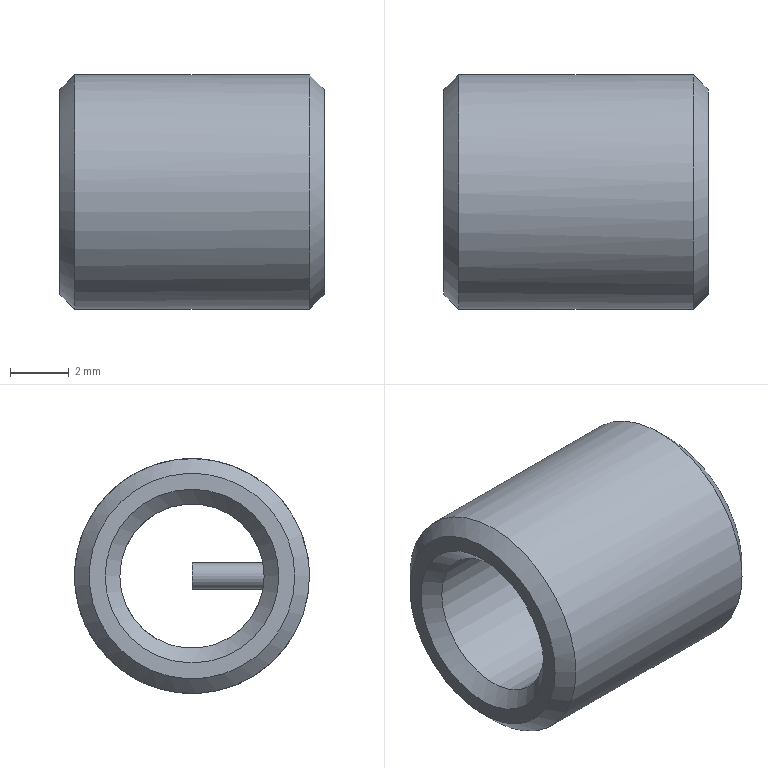Part | STEP file | Part [3] | 1 solid | 10 faces | box 9 x 8 x 8 mm | volume 272.983 mm3 | cone 4 | plane 3 | cylinder 3 | commonest cylinder face diameters 0.9 x1 4.917 x1 8 x1
STEP:
#1=CARTESIAN_POINT('',(13.5,104.,0.));
#2=VERTEX_POINT('',#1);
#3=CARTESIAN_POINT('',(13.5,107.5,0.));
#4=DIRECTION('',(1.,0.,0.));
#5=DIRECTION('',(0.,0.,1.));
#6=AXIS2_PLACEMENT_3D('',#3,#4,#5);
#7=CIRCLE('',#6,3.5);
#8=EDGE_CURVE('',#2,#2,#7,.T.);
#9=ORIENTED_EDGE('',*,*,#8,.F.);
#10=EDGE_LOOP('',(#9));
#11=FACE_BOUND('',#10,.T.);
#12=CARTESIAN_POINT('',(13.5,104.541,0.));
#13=VERTEX_POINT('',#12);
#14=CARTESIAN_POINT('',(13.5,107.5,0.));
#15=DIRECTION('',(1.,0.,0.));
#16=DIRECTION('',(0.,0.,1.));
#17=AXIS2_PLACEMENT_3D('',#14,#15,#16);
#18=CIRCLE('',#17,2.958);
#19=EDGE_CURVE('',#13,#13,#18,.T.);
#20=ORIENTED_EDGE('',*,*,#19,.T.);
#21=EDGE_LOOP('',(#20));
#22=FACE_BOUND('',#21,.T.);
#23=CARTESIAN_POINT('',(13.5,107.5,0.));
#24=DIRECTION('',(1.,0.,0.));
#25=DIRECTION('',(0.,0.,1.));
#26=AXIS2_PLACEMENT_3D('',#23,#24,#25);
#27=PLANE('',#26);
#28=ADVANCED_FACE('',(#11,#22),#27,.F.);
#29=CARTESIAN_POINT('',(14.,103.5,0.));
#30=VERTEX_POINT('',#29);
#31=CARTESIAN_POINT('',(14.,103.5,0.));
#32=CARTESIAN_POINT('',(14.,103.5,-0.08379));
#33=CARTESIAN_POINT('',(14.,103.505,-0.2514));
#34=CARTESIAN_POINT('',(14.,103.529,-0.5017));
#35=CARTESIAN_POINT('',(14.,103.568,-0.7501));
#36=CARTESIAN_POINT('',(14.,103.623,-0.9956));
#37=CARTESIAN_POINT('',(14.,103.693,-1.237));
#38=CARTESIAN_POINT('',(14.,103.779,-1.474));
#39=CARTESIAN_POINT('',(14.,103.878,-1.704));
#40=CARTESIAN_POINT('',(14.,103.993,-1.929));
#41=CARTESIAN_POINT('',(14.,104.121,-2.145));
#42=CARTESIAN_POINT('',(14.,104.262,-2.353));
#43=CARTESIAN_POINT('',(14.,104.416,-2.552));
#44=CARTESIAN_POINT('',(14.,104.583,-2.74));
#45=CARTESIAN_POINT('',(14.,104.76,-2.918));
#46=CARTESIAN_POINT('',(14.,104.949,-3.084));
#47=CARTESIAN_POINT('',(14.,105.148,-3.239));
#48=CARTESIAN_POINT('',(14.,105.356,-3.38));
#49=CARTESIAN_POINT('',(14.,105.572,-3.508));
#50=CARTESIAN_POINT('',(14.,105.796,-3.622));
#51=CARTESIAN_POINT('',(14.,106.027,-3.722));
#52=CARTESIAN_POINT('',(14.,106.264,-3.807));
#53=CARTESIAN_POINT('',(14.,106.505,-3.877));
#54=CARTESIAN_POINT('',(14.,106.751,-3.932));
#55=CARTESIAN_POINT('',(14.,106.999,-3.971));
#56=CARTESIAN_POINT('',(14.,107.25,-3.995));
#57=CARTESIAN_POINT('',(14.,107.501,-4.003));
#58=CARTESIAN_POINT('',(14.,107.752,-3.995));
#59=CARTESIAN_POINT('',(14.,108.003,-3.971));
#60=CARTESIAN_POINT('',(14.,108.251,-3.932));
#61=CARTESIAN_POINT('',(14.,108.497,-3.877));
#62=CARTESIAN_POINT('',(14.,108.738,-3.806));
#63=CARTESIAN_POINT('',(14.,108.975,-3.721));
#64=CARTESIAN_POINT('',(14.,109.205,-3.621));
#65=CARTESIAN_POINT('',(14.,109.429,-3.507));
#66=CARTESIAN_POINT('',(14.,109.646,-3.379));
#67=CARTESIAN_POINT('',(14.,109.854,-3.237));
#68=CARTESIAN_POINT('',(14.,110.052,-3.083));
#69=CARTESIAN_POINT('',(14.,110.241,-2.917));
#70=CARTESIAN_POINT('',(14.,110.419,-2.739));
#71=CARTESIAN_POINT('',(14.,110.585,-2.55));
#72=CARTESIAN_POINT('',(14.,110.739,-2.351));
#73=CARTESIAN_POINT('',(14.,110.88,-2.143));
#74=CARTESIAN_POINT('',(14.,111.008,-1.927));
#75=CARTESIAN_POINT('',(14.,111.122,-1.703));
#76=CARTESIAN_POINT('',(14.,111.222,-1.472));
#77=CARTESIAN_POINT('',(14.,111.307,-1.235));
#78=CARTESIAN_POINT('',(14.,111.377,-0.9936));
#79=CARTESIAN_POINT('',(14.,111.432,-0.7482));
#80=CARTESIAN_POINT('',(14.,111.471,-0.4998));
#81=CARTESIAN_POINT('',(14.,111.495,-0.25));
#82=CARTESIAN_POINT('',(14.,111.5,-0.08312));
#83=CARTESIAN_POINT('',(14.,111.5,0.));
#84=CARTESIAN_POINT('',(14.,111.5,0.08379));
#85=CARTESIAN_POINT('',(14.,111.495,0.2514));
#86=CARTESIAN_POINT('',(14.,111.471,0.5017));
#87=CARTESIAN_POINT('',(14.,111.432,0.7501));
#88=CARTESIAN_POINT('',(14.,111.377,0.9956));
#89=CARTESIAN_POINT('',(14.,111.307,1.237));
#90=CARTESIAN_POINT('',(14.,111.221,1.474));
#91=CARTESIAN_POINT('',(14.,111.122,1.704));
#92=CARTESIAN_POINT('',(14.,111.007,1.929));
#93=CARTESIAN_POINT('',(14.,110.879,2.145));
#94=CARTESIAN_POINT('',(14.,110.738,2.353));
#95=CARTESIAN_POINT('',(14.,110.584,2.552));
#96=CARTESIAN_POINT('',(14.,110.417,2.74));
#97=CARTESIAN_POINT('',(14.,110.24,2.918));
#98=CARTESIAN_POINT('',(14.,110.051,3.084));
#99=CARTESIAN_POINT('',(14.,109.852,3.239));
#100=CARTESIAN_POINT('',(14.,109.644,3.38));
#101=CARTESIAN_POINT('',(14.,109.428,3.508));
#102=CARTESIAN_POINT('',(14.,109.204,3.622));
#103=CARTESIAN_POINT('',(14.,108.973,3.722));
#104=CARTESIAN_POINT('',(14.,108.736,3.807));
#105=CARTESIAN_POINT('',(14.,108.495,3.877));
#106=CARTESIAN_POINT('',(14.,108.249,3.932));
#107=CARTESIAN_POINT('',(14.,108.001,3.971));
#108=CARTESIAN_POINT('',(14.,107.75,3.995));
#109=CARTESIAN_POINT('',(14.,107.499,4.003));
#110=CARTESIAN_POINT('',(14.,107.248,3.995));
#111=CARTESIAN_POINT('',(14.,106.997,3.971));
#112=CARTESIAN_POINT('',(14.,106.749,3.932));
#113=CARTESIAN_POINT('',(14.,106.503,3.877));
#114=CARTESIAN_POINT('',(14.,106.262,3.806));
#115=CARTESIAN_POINT('',(14.,106.025,3.721));
#116=CARTESIAN_POINT('',(14.,105.795,3.621));
#117=CARTESIAN_POINT('',(14.,105.571,3.507));
#118=CARTESIAN_POINT('',(14.,105.354,3.379));
#119=CARTESIAN_POINT('',(14.,105.146,3.237));
#120=CARTESIAN_POINT('',(14.,104.948,3.083));
#121=CARTESIAN_POINT('',(14.,104.759,2.917));
#122=CARTESIAN_POINT('',(14.,104.581,2.739));
#123=CARTESIAN_POINT('',(14.,104.415,2.55));
#124=CARTESIAN_POINT('',(14.,104.261,2.351));
#125=CARTESIAN_POINT('',(14.,104.12,2.143));
#126=CARTESIAN_POINT('',(14.,103.992,1.927));
#127=CARTESIAN_POINT('',(14.,103.878,1.703));
#128=CARTESIAN_POINT('',(14.,103.778,1.472));
#129=CARTESIAN_POINT('',(14.,103.693,1.235));
#130=CARTESIAN_POINT('',(14.,103.623,0.9936));
#131=CARTESIAN_POINT('',(14.,103.568,0.7482));
#132=CARTESIAN_POINT('',(14.,103.529,0.4998));
#133=CARTESIAN_POINT('',(14.,103.505,0.25));
#134=CARTESIAN_POINT('',(14.,103.5,0.08312));
#135=CARTESIAN_POINT('',(14.,103.5,0.));
#136=B_SPLINE_CURVE_WITH_KNOTS('',3,(#31,#32,#33,#34,#35,#36,#37,#38,#39,#40,#41,#42,#43,#44,#45,#46,#47,#48,#49,#50,#51,#52,#53,#54,#55,#56,#57,#58,#59,#60,#61,#62,#63,#64,#65,#66,#67,#68,#69,#70,#71,#72,#73,#74,#75,#76,#77,#78,#79,#80,#81,#82,#83,#84,#85,#86,#87,#88,#89,#90,#91,#92,#93,#94,#95,#96,#97,#98,#99,#100,#101,#102,#103,#104,#105,#106,#107,#108,#109,#110,#111,#112,#113,#114,#115,#116,#117,#118,#119,#120,#121,#122,#123,#124,#125,#126,#127,#128,#129,#130,#131,#132,#133,#134,#135),.UNSPECIFIED.,.T.,.F.,(4,1,1,1,1,1,1,1,1,1,1,1,1,1,1,1,1,1,1,1,1,1,1,1,1,1,1,1,1,1,1,1,1,1,1,1,1,1,1,1,1,1,1,1,1,1,1,1,1,1,3,1,1,1,1,1,1,1,1,1,1,1,1,1,1,1,1,1,1,1,1,1,1,1,1,1,1,1,1,1,1,1,1,1,1,1,1,1,1,1,1,1,1,1,1,1,1,1,1,1,4),(0.,0.01,0.02,0.03,0.04001,0.05001,0.06001,0.07001,0.08001,0.09001,0.1,0.11,0.12,0.13,0.14,0.15,0.16,0.17,0.18,0.19,0.2,0.21,0.22,0.23,0.24,0.25,0.26,0.27,0.28,0.29,0.3,0.31,0.3201,0.3301,0.3401,0.3501,0.3601,0.3701,0.3801,0.3901,0.4001,0.4101,0.4201,0.4301,0.4401,0.4501,0.4601,0.4701,0.4801,0.4901,0.5,0.51,0.52,0.53,0.54,0.55,0.56,0.57,0.58,0.59,0.6,0.61,0.62,0.63,0.64,0.65,0.66,0.67,0.68,0.69,0.7,0.71,0.72,0.73,0.74,0.75,0.76,0.77,0.78,0.79,0.8,0.81,0.8201,0.8301,0.8401,0.8501,0.8601,0.8701,0.8801,0.8901,0.9001,0.9101,0.9201,0.9301,0.9401,0.9501,0.9601,0.9701,0.9801,0.9901,1.),.UNSPECIFIED.);
#137=EDGE_CURVE('',#30,#30,#136,.T.);
#138=ORIENTED_EDGE('',*,*,#137,.F.);
#139=EDGE_LOOP('',(#138));
#140=FACE_OUTER_BOUND('',#139,.T.);
#141=ORIENTED_EDGE('',*,*,#8,.T.);
#142=EDGE_LOOP('',(#141));
#143=FACE_OUTER_BOUND('',#142,.T.);
#144=CARTESIAN_POINT('',(13.75,107.5,0.));
#145=DIRECTION('',(1.,0.,0.));
#146=DIRECTION('',(0.,-1.,0.));
#147=AXIS2_PLACEMENT_3D('',#144,#145,#146);
#148=CONICAL_SURFACE('',#147,3.75,0.7854);
#149=ADVANCED_FACE('',(#140,#143),#148,.T.);
#150=CARTESIAN_POINT('',(22.,103.5,0.));
#151=VERTEX_POINT('',#150);
#152=CARTESIAN_POINT('',(22.,111.5,0.));
#153=VERTEX_POINT('',#152);
#154=CARTESIAN_POINT('',(22.,107.5,0.));
#155=DIRECTION('',(1.,0.,0.));
#156=DIRECTION('',(0.,-1.,0.));
#157=AXIS2_PLACEMENT_3D('',#154,#155,#156);
#158=CIRCLE('',#157,4.);
#159=EDGE_CURVE('',#151,#153,#158,.T.);
#160=ORIENTED_EDGE('',*,*,#159,.F.);
#161=CARTESIAN_POINT('',(22.,107.5,0.));
#162=DIRECTION('',(1.,0.,0.));
#163=DIRECTION('',(0.,1.,0.));
#164=AXIS2_PLACEMENT_3D('',#161,#162,#163);
#165=CIRCLE('',#164,4.);
#166=EDGE_CURVE('',#153,#151,#165,.T.);
#167=ORIENTED_EDGE('',*,*,#166,.F.);
#168=EDGE_LOOP('',(#160,#167));
#169=FACE_BOUND('',#168,.T.);
#170=ORIENTED_EDGE('',*,*,#137,.T.);
#171=EDGE_LOOP('',(#170));
#172=FACE_OUTER_BOUND('',#171,.T.);
#173=CARTESIAN_POINT('',(13.5,107.5,0.));
#174=DIRECTION('',(1.,0.,0.));
#175=DIRECTION('',(0.,-1.,0.));
#176=AXIS2_PLACEMENT_3D('',#173,#174,#175);
#177=CYLINDRICAL_SURFACE('',#176,4.);
#178=ADVANCED_FACE('',(#169,#172),#177,.T.);
#179=CARTESIAN_POINT('',(22.5,111.,0.));
#180=VERTEX_POINT('',#179);
#181=CARTESIAN_POINT('',(22.5,107.5,0.));
#182=DIRECTION('',(1.,0.,0.));
#183=DIRECTION('',(0.,0.,1.));
#184=AXIS2_PLACEMENT_3D('',#181,#182,#183);
#185=CIRCLE('',#184,3.5);
#186=EDGE_CURVE('',#180,#180,#185,.T.);
#187=ORIENTED_EDGE('',*,*,#186,.F.);
#188=EDGE_LOOP('',(#187));
#189=FACE_OUTER_BOUND('',#188,.T.);
#190=ORIENTED_EDGE('',*,*,#166,.T.);
#191=ORIENTED_EDGE('',*,*,#159,.T.);
#192=EDGE_LOOP('',(#190,#191));
#193=FACE_BOUND('',#192,.T.);
#194=CARTESIAN_POINT('',(22.25,107.5,0.));
#195=DIRECTION('',(-1.,0.,0.));
#196=DIRECTION('',(0.,-1.,0.));
#197=AXIS2_PLACEMENT_3D('',#194,#195,#196);
#198=CONICAL_SURFACE('',#197,3.75,0.7854);
#199=ADVANCED_FACE('',(#189,#193),#198,.T.);
#200=ORIENTED_EDGE('',*,*,#186,.T.);
#201=EDGE_LOOP('',(#200));
#202=FACE_BOUND('',#201,.T.);
#203=CARTESIAN_POINT('',(22.5,104.541,0.));
#204=VERTEX_POINT('',#203);
#205=CARTESIAN_POINT('',(22.5,107.5,0.));
#206=DIRECTION('',(1.,0.,0.));
#207=DIRECTION('',(0.,0.,1.));
#208=AXIS2_PLACEMENT_3D('',#205,#206,#207);
#209=CIRCLE('',#208,2.958);
#210=EDGE_CURVE('',#204,#204,#209,.T.);
#211=ORIENTED_EDGE('',*,*,#210,.F.);
#212=EDGE_LOOP('',(#211));
#213=FACE_BOUND('',#212,.T.);
#214=CARTESIAN_POINT('',(22.5,107.5,0.));
#215=DIRECTION('',(1.,0.,0.));
#216=DIRECTION('',(0.,0.,1.));
#217=AXIS2_PLACEMENT_3D('',#214,#215,#216);
#218=PLANE('',#217);
#219=ADVANCED_FACE('',(#202,#213),#218,.T.);
#220=CARTESIAN_POINT('',(22.,105.083,-0.4472));
#221=VERTEX_POINT('',#220);
#222=CARTESIAN_POINT('',(22.,109.959,0.));
#223=VERTEX_POINT('',#222);
#224=CARTESIAN_POINT('',(22.,107.5,0.));
#225=DIRECTION('',(1.,0.,0.));
#226=DIRECTION('',(0.,-0.9833,-0.1819));
#227=AXIS2_PLACEMENT_3D('',#224,#225,#226);
#228=CIRCLE('',#227,2.458);
#229=EDGE_CURVE('',#221,#223,#228,.T.);
#230=ORIENTED_EDGE('',*,*,#229,.F.);
#231=CARTESIAN_POINT('',(22.5,104.541,0.));
#232=CARTESIAN_POINT('',(22.5,104.541,-0.002951));
#233=CARTESIAN_POINT('',(22.5,104.542,-0.009389));
#234=CARTESIAN_POINT('',(22.5,104.542,-0.01991));
#235=CARTESIAN_POINT('',(22.499,104.543,-0.03476));
#236=CARTESIAN_POINT('',(22.497,104.545,-0.0564));
#237=CARTESIAN_POINT('',(22.492,104.551,-0.08654));
#238=CARTESIAN_POINT('',(22.484,104.559,-0.1189));
#239=CARTESIAN_POINT('',(22.476,104.57,-0.1471));
#240=CARTESIAN_POINT('',(22.468,104.578,-0.1663));
#241=CARTESIAN_POINT('',(22.463,104.584,-0.1795));
#242=CARTESIAN_POINT('',(22.458,104.59,-0.1908));
#243=CARTESIAN_POINT('',(22.452,104.597,-0.2027));
#244=CARTESIAN_POINT('',(22.445,104.604,-0.2149));
#245=CARTESIAN_POINT('',(22.439,104.611,-0.2259));
#246=CARTESIAN_POINT('',(22.433,104.618,-0.2357));
#247=CARTESIAN_POINT('',(22.428,104.624,-0.2443));
#248=CARTESIAN_POINT('',(22.422,104.63,-0.2528));
#249=CARTESIAN_POINT('',(22.416,104.637,-0.2614));
#250=CARTESIAN_POINT('',(22.41,104.645,-0.2704));
#251=CARTESIAN_POINT('',(22.401,104.654,-0.2813));
#252=CARTESIAN_POINT('',(22.391,104.665,-0.2936));
#253=CARTESIAN_POINT('',(22.379,104.679,-0.3068));
#254=CARTESIAN_POINT('',(22.367,104.692,-0.3191));
#255=CARTESIAN_POINT('',(22.356,104.705,-0.3303));
#256=CARTESIAN_POINT('',(22.345,104.717,-0.3402));
#257=CARTESIAN_POINT('',(22.335,104.729,-0.3486));
#258=CARTESIAN_POINT('',(22.325,104.739,-0.3559));
#259=CARTESIAN_POINT('',(22.317,104.748,-0.3624));
#260=CARTESIAN_POINT('',(22.308,104.758,-0.3689));
#261=CARTESIAN_POINT('',(22.298,104.769,-0.3752));
#262=CARTESIAN_POINT('',(22.289,104.779,-0.3815));
#263=CARTESIAN_POINT('',(22.279,104.79,-0.3876));
#264=CARTESIAN_POINT('',(22.268,104.802,-0.3936));
#265=CARTESIAN_POINT('',(22.257,104.814,-0.3995));
#266=CARTESIAN_POINT('',(22.246,104.826,-0.4051));
#267=CARTESIAN_POINT('',(22.234,104.839,-0.4106));
#268=CARTESIAN_POINT('',(22.222,104.851,-0.4157));
#269=CARTESIAN_POINT('',(22.21,104.865,-0.4206));
#270=CARTESIAN_POINT('',(22.198,104.878,-0.4251));
#271=CARTESIAN_POINT('',(22.185,104.891,-0.4293));
#272=CARTESIAN_POINT('',(22.172,104.905,-0.4331));
#273=CARTESIAN_POINT('',(22.16,104.918,-0.4365));
#274=CARTESIAN_POINT('',(22.147,104.932,-0.4395));
#275=CARTESIAN_POINT('',(22.135,104.945,-0.442));
#276=CARTESIAN_POINT('',(22.123,104.957,-0.4441));
#277=CARTESIAN_POINT('',(22.111,104.97,-0.4459));
#278=CARTESIAN_POINT('',(22.1,104.981,-0.4473));
#279=CARTESIAN_POINT('',(22.089,104.993,-0.4484));
#280=CARTESIAN_POINT('',(22.078,105.004,-0.4492));
#281=CARTESIAN_POINT('',(22.068,105.014,-0.4497));
#282=CARTESIAN_POINT('',(22.058,105.024,-0.45));
#283=CARTESIAN_POINT('',(22.052,105.031,-0.45));
#284=CARTESIAN_POINT('',(22.045,105.037,-0.45));
#285=CARTESIAN_POINT('',(22.038,105.045,-0.4499));
#286=CARTESIAN_POINT('',(22.028,105.054,-0.4495));
#287=CARTESIAN_POINT('',(22.019,105.064,-0.4489));
#288=CARTESIAN_POINT('',(22.009,105.073,-0.4482));
#289=CARTESIAN_POINT('',(22.003,105.079,-0.4476));
#290=CARTESIAN_POINT('',(22.,105.083,-0.4472));
#291=B_SPLINE_CURVE_WITH_KNOTS('',3,(#231,#232,#233,#234,#235,#236,#237,#238,#239,#240,#241,#242,#243,#244,#245,#246,#247,#248,#249,#250,#251,#252,#253,#254,#255,#256,#257,#258,#259,#260,#261,#262,#263,#264,#265,#266,#267,#268,#269,#270,#271,#272,#273,#274,#275,#276,#277,#278,#279,#280,#281,#282,#283,#284,#285,#286,#287,#288,#289,#290),.UNSPECIFIED.,.F.,.F.,(4,1,1,1,1,1,1,1,1,1,1,1,1,1,1,1,1,1,1,1,1,1,1,1,1,1,1,1,1,1,1,1,1,1,1,1,1,1,1,1,1,1,1,1,1,1,1,1,1,1,1,1,1,1,1,1,1,4),(0.,0.01496,0.0325,0.05264,0.08847,0.1383,0.1977,0.2424,0.2713,0.2883,0.3049,0.3251,0.3449,0.3641,0.3785,0.3929,0.4071,0.4212,0.4367,0.4537,0.4784,0.503,0.5275,0.549,0.569,0.5874,0.6012,0.6152,0.6294,0.6436,0.6581,0.6727,0.6874,0.7022,0.7172,0.7323,0.7474,0.7625,0.7777,0.7928,0.8078,0.8226,0.8369,0.851,0.8645,0.8778,0.8904,0.9025,0.9141,0.9255,0.9366,0.9447,0.9476,0.9582,0.9688,0.9792,0.9896,1.),.UNSPECIFIED.);
#292=EDGE_CURVE('',#204,#221,#291,.T.);
#293=ORIENTED_EDGE('',*,*,#292,.F.);
#294=ORIENTED_EDGE('',*,*,#210,.T.);
#295=CARTESIAN_POINT('',(22.,105.083,0.4472));
#296=VERTEX_POINT('',#295);
#297=CARTESIAN_POINT('',(22.5,104.541,0.));
#298=CARTESIAN_POINT('',(22.5,104.541,0.002951));
#299=CARTESIAN_POINT('',(22.5,104.542,0.009389));
#300=CARTESIAN_POINT('',(22.5,104.542,0.01991));
#301=CARTESIAN_POINT('',(22.499,104.543,0.03476));
#302=CARTESIAN_POINT('',(22.497,104.545,0.0564));
#303=CARTESIAN_POINT('',(22.492,104.551,0.08654));
#304=CARTESIAN_POINT('',(22.484,104.559,0.1189));
#305=CARTESIAN_POINT('',(22.476,104.57,0.1471));
#306=CARTESIAN_POINT('',(22.468,104.578,0.1663));
#307=CARTESIAN_POINT('',(22.463,104.584,0.1795));
#308=CARTESIAN_POINT('',(22.458,104.59,0.1908));
#309=CARTESIAN_POINT('',(22.452,104.597,0.2027));
#310=CARTESIAN_POINT('',(22.445,104.604,0.2149));
#311=CARTESIAN_POINT('',(22.439,104.611,0.2259));
#312=CARTESIAN_POINT('',(22.433,104.618,0.2357));
#313=CARTESIAN_POINT('',(22.428,104.624,0.2443));
#314=CARTESIAN_POINT('',(22.422,104.63,0.2528));
#315=CARTESIAN_POINT('',(22.416,104.637,0.2614));
#316=CARTESIAN_POINT('',(22.41,104.645,0.2704));
#317=CARTESIAN_POINT('',(22.401,104.654,0.2813));
#318=CARTESIAN_POINT('',(22.391,104.665,0.2936));
#319=CARTESIAN_POINT('',(22.379,104.679,0.3068));
#320=CARTESIAN_POINT('',(22.367,104.692,0.3191));
#321=CARTESIAN_POINT('',(22.356,104.705,0.3303));
#322=CARTESIAN_POINT('',(22.345,104.717,0.3402));
#323=CARTESIAN_POINT('',(22.335,104.729,0.3486));
#324=CARTESIAN_POINT('',(22.325,104.739,0.3559));
#325=CARTESIAN_POINT('',(22.317,104.748,0.3624));
#326=CARTESIAN_POINT('',(22.308,104.758,0.3689));
#327=CARTESIAN_POINT('',(22.298,104.769,0.3752));
#328=CARTESIAN_POINT('',(22.289,104.779,0.3815));
#329=CARTESIAN_POINT('',(22.279,104.79,0.3876));
#330=CARTESIAN_POINT('',(22.268,104.802,0.3936));
#331=CARTESIAN_POINT('',(22.257,104.814,0.3995));
#332=CARTESIAN_POINT('',(22.246,104.826,0.4051));
#333=CARTESIAN_POINT('',(22.234,104.839,0.4106));
#334=CARTESIAN_POINT('',(22.222,104.851,0.4157));
#335=CARTESIAN_POINT('',(22.21,104.865,0.4206));
#336=CARTESIAN_POINT('',(22.198,104.878,0.4251));
#337=CARTESIAN_POINT('',(22.185,104.891,0.4293));
#338=CARTESIAN_POINT('',(22.172,104.905,0.4331));
#339=CARTESIAN_POINT('',(22.16,104.918,0.4365));
#340=CARTESIAN_POINT('',(22.147,104.932,0.4395));
#341=CARTESIAN_POINT('',(22.135,104.945,0.442));
#342=CARTESIAN_POINT('',(22.123,104.957,0.4441));
#343=CARTESIAN_POINT('',(22.111,104.97,0.4459));
#344=CARTESIAN_POINT('',(22.1,104.981,0.4473));
#345=CARTESIAN_POINT('',(22.089,104.993,0.4484));
#346=CARTESIAN_POINT('',(22.078,105.004,0.4492));
#347=CARTESIAN_POINT('',(22.068,105.014,0.4497));
#348=CARTESIAN_POINT('',(22.058,105.024,0.45));
#349=CARTESIAN_POINT('',(22.052,105.031,0.45));
#350=CARTESIAN_POINT('',(22.045,105.037,0.45));
#351=CARTESIAN_POINT('',(22.038,105.045,0.4499));
#352=CARTESIAN_POINT('',(22.028,105.054,0.4495));
#353=CARTESIAN_POINT('',(22.019,105.064,0.4489));
#354=CARTESIAN_POINT('',(22.009,105.073,0.4482));
#355=CARTESIAN_POINT('',(22.003,105.079,0.4476));
#356=CARTESIAN_POINT('',(22.,105.083,0.4472));
#357=B_SPLINE_CURVE_WITH_KNOTS('',3,(#297,#298,#299,#300,#301,#302,#303,#304,#305,#306,#307,#308,#309,#310,#311,#312,#313,#314,#315,#316,#317,#318,#319,#320,#321,#322,#323,#324,#325,#326,#327,#328,#329,#330,#331,#332,#333,#334,#335,#336,#337,#338,#339,#340,#341,#342,#343,#344,#345,#346,#347,#348,#349,#350,#351,#352,#353,#354,#355,#356),.UNSPECIFIED.,.F.,.F.,(4,1,1,1,1,1,1,1,1,1,1,1,1,1,1,1,1,1,1,1,1,1,1,1,1,1,1,1,1,1,1,1,1,1,1,1,1,1,1,1,1,1,1,1,1,1,1,1,1,1,1,1,1,1,1,1,1,4),(0.,0.01496,0.0325,0.05264,0.08847,0.1383,0.1977,0.2424,0.2713,0.2883,0.3049,0.3252,0.3449,0.3641,0.3785,0.3929,0.4071,0.4212,0.4367,0.4537,0.4784,0.503,0.5275,0.549,0.569,0.5874,0.6012,0.6152,0.6294,0.6436,0.6581,0.6727,0.6874,0.7022,0.7172,0.7323,0.7474,0.7625,0.7777,0.7928,0.8078,0.8226,0.8369,0.851,0.8645,0.8778,0.8904,0.9025,0.9141,0.9255,0.9366,0.9447,0.9476,0.9582,0.9688,0.9792,0.9896,1.),.UNSPECIFIED.);
#358=EDGE_CURVE('',#204,#296,#357,.T.);
#359=ORIENTED_EDGE('',*,*,#358,.T.);
#360=CARTESIAN_POINT('',(22.,107.5,0.));
#361=DIRECTION('',(1.,0.,0.));
#362=DIRECTION('',(0.,1.,0.));
#363=AXIS2_PLACEMENT_3D('',#360,#361,#362);
#364=CIRCLE('',#363,2.458);
#365=EDGE_CURVE('',#223,#296,#364,.T.);
#366=ORIENTED_EDGE('',*,*,#365,.F.);
#367=EDGE_LOOP('',(#230,#293,#294,#359,#366));
#368=FACE_BOUND('',#367,.T.);
#369=CARTESIAN_POINT('',(22.25,107.5,0.));
#370=DIRECTION('',(1.,0.,0.));
#371=DIRECTION('',(0.,-1.,0.));
#372=AXIS2_PLACEMENT_3D('',#369,#370,#371);
#373=CONICAL_SURFACE('',#372,2.708,0.7854);
#374=ADVANCED_FACE('',(#368),#373,.F.);
#375=ORIENTED_EDGE('',*,*,#292,.T.);
#376=CARTESIAN_POINT('',(21.6,105.041,0.));
#377=VERTEX_POINT('',#376);
#378=CARTESIAN_POINT('',(22.,105.083,-0.4472));
#379=CARTESIAN_POINT('',(21.991,105.082,-0.4462));
#380=CARTESIAN_POINT('',(21.972,105.082,-0.4435));
#381=CARTESIAN_POINT('',(21.945,105.081,-0.4378));
#382=CARTESIAN_POINT('',(21.918,105.079,-0.4304));
#383=CARTESIAN_POINT('',(21.891,105.078,-0.4214));
#384=CARTESIAN_POINT('',(21.865,105.076,-0.4106));
#385=CARTESIAN_POINT('',(21.84,105.074,-0.3982));
#386=CARTESIAN_POINT('',(21.815,105.072,-0.3842));
#387=CARTESIAN_POINT('',(21.791,105.069,-0.3687));
#388=CARTESIAN_POINT('',(21.766,105.066,-0.3498));
#389=CARTESIAN_POINT('',(21.74,105.063,-0.3271));
#390=CARTESIAN_POINT('',(21.714,105.06,-0.3002));
#391=CARTESIAN_POINT('',(21.692,105.057,-0.2735));
#392=CARTESIAN_POINT('',(21.674,105.054,-0.2477));
#393=CARTESIAN_POINT('',(21.657,105.051,-0.2207));
#394=CARTESIAN_POINT('',(21.641,105.049,-0.1893));
#395=CARTESIAN_POINT('',(21.626,105.046,-0.1531));
#396=CARTESIAN_POINT('',(21.615,105.044,-0.1186));
#397=CARTESIAN_POINT('',(21.608,105.043,-0.08754));
#398=CARTESIAN_POINT('',(21.604,105.042,-0.06193));
#399=CARTESIAN_POINT('',(21.602,105.042,-0.03905));
#400=CARTESIAN_POINT('',(21.6,105.042,-0.01887));
#401=CARTESIAN_POINT('',(21.6,105.042,-0.006058));
#402=CARTESIAN_POINT('',(21.6,105.041,0.));
#403=B_SPLINE_CURVE_WITH_KNOTS('',3,(#378,#379,#380,#381,#382,#383,#384,#385,#386,#387,#388,#389,#390,#391,#392,#393,#394,#395,#396,#397,#398,#399,#400,#401,#402),.UNSPECIFIED.,.F.,.F.,(4,1,1,1,1,1,1,1,1,1,1,1,1,1,1,1,1,1,1,1,1,1,4),(0.,0.04241,0.08488,0.1273,0.1697,0.2121,0.2546,0.2972,0.3403,0.3835,0.4418,0.5002,0.5589,0.6025,0.6459,0.703,0.7616,0.8216,0.8657,0.9066,0.941,0.9722,1.),.UNSPECIFIED.);
#404=EDGE_CURVE('',#221,#377,#403,.T.);
#405=ORIENTED_EDGE('',*,*,#404,.T.);
#406=CARTESIAN_POINT('',(21.6,105.041,0.));
#407=CARTESIAN_POINT('',(21.6,105.041,0.002689));
#408=CARTESIAN_POINT('',(21.6,105.042,0.008077));
#409=CARTESIAN_POINT('',(21.6,105.042,0.01618));
#410=CARTESIAN_POINT('',(21.601,105.042,0.02431));
#411=CARTESIAN_POINT('',(21.601,105.042,0.03247));
#412=CARTESIAN_POINT('',(21.602,105.042,0.04068));
#413=CARTESIAN_POINT('',(21.603,105.042,0.04894));
#414=CARTESIAN_POINT('',(21.604,105.042,0.05729));
#415=CARTESIAN_POINT('',(21.605,105.042,0.06569));
#416=CARTESIAN_POINT('',(21.606,105.043,0.07416));
#417=CARTESIAN_POINT('',(21.608,105.043,0.0827));
#418=CARTESIAN_POINT('',(21.609,105.043,0.09134));
#419=CARTESIAN_POINT('',(21.611,105.044,0.1));
#420=CARTESIAN_POINT('',(21.613,105.044,0.1088));
#421=CARTESIAN_POINT('',(21.616,105.044,0.1177));
#422=CARTESIAN_POINT('',(21.618,105.045,0.1266));
#423=CARTESIAN_POINT('',(21.621,105.045,0.1356));
#424=CARTESIAN_POINT('',(21.624,105.046,0.1449));
#425=CARTESIAN_POINT('',(21.627,105.046,0.1549));
#426=CARTESIAN_POINT('',(21.632,105.047,0.1672));
#427=CARTESIAN_POINT('',(21.639,105.048,0.1829));
#428=CARTESIAN_POINT('',(21.648,105.05,0.2022));
#429=CARTESIAN_POINT('',(21.658,105.051,0.2215));
#430=CARTESIAN_POINT('',(21.668,105.053,0.2378));
#431=CARTESIAN_POINT('',(21.676,105.054,0.2498));
#432=CARTESIAN_POINT('',(21.682,105.055,0.2591));
#433=CARTESIAN_POINT('',(21.688,105.056,0.2673));
#434=CARTESIAN_POINT('',(21.694,105.057,0.2753));
#435=CARTESIAN_POINT('',(21.701,105.058,0.2836));
#436=CARTESIAN_POINT('',(21.708,105.059,0.2925));
#437=CARTESIAN_POINT('',(21.718,105.06,0.3039));
#438=CARTESIAN_POINT('',(21.732,105.062,0.3189));
#439=CARTESIAN_POINT('',(21.751,105.065,0.3364));
#440=CARTESIAN_POINT('',(21.77,105.067,0.3529));
#441=CARTESIAN_POINT('',(21.787,105.069,0.3656));
#442=CARTESIAN_POINT('',(21.801,105.07,0.375));
#443=CARTESIAN_POINT('',(21.815,105.072,0.3838));
#444=CARTESIAN_POINT('',(21.832,105.073,0.394));
#445=CARTESIAN_POINT('',(21.853,105.075,0.405));
#446=CARTESIAN_POINT('',(21.874,105.077,0.4145));
#447=CARTESIAN_POINT('',(21.892,105.078,0.4213));
#448=CARTESIAN_POINT('',(21.904,105.079,0.4259));
#449=CARTESIAN_POINT('',(21.914,105.079,0.4291));
#450=CARTESIAN_POINT('',(21.924,105.08,0.4319));
#451=CARTESIAN_POINT('',(21.932,105.08,0.4344));
#452=CARTESIAN_POINT('',(21.941,105.081,0.4368));
#453=CARTESIAN_POINT('',(21.951,105.081,0.439));
#454=CARTESIAN_POINT('',(21.96,105.081,0.441));
#455=CARTESIAN_POINT('',(21.97,105.082,0.4429));
#456=CARTESIAN_POINT('',(21.98,105.082,0.4445));
#457=CARTESIAN_POINT('',(21.99,105.082,0.446));
#458=CARTESIAN_POINT('',(21.997,105.082,0.4468));
#459=CARTESIAN_POINT('',(22.,105.083,0.4472));
#460=B_SPLINE_CURVE_WITH_KNOTS('',3,(#406,#407,#408,#409,#410,#411,#412,#413,#414,#415,#416,#417,#418,#419,#420,#421,#422,#423,#424,#425,#426,#427,#428,#429,#430,#431,#432,#433,#434,#435,#436,#437,#438,#439,#440,#441,#442,#443,#444,#445,#446,#447,#448,#449,#450,#451,#452,#453,#454,#455,#456,#457,#458,#459),.UNSPECIFIED.,.F.,.F.,(4,1,1,1,1,1,1,1,1,1,1,1,1,1,1,1,1,1,1,1,1,1,1,1,1,1,1,1,1,1,1,1,1,1,1,1,1,1,1,1,1,1,1,1,1,1,1,1,1,1,1,4),(0.,0.01247,0.02497,0.03749,0.05008,0.0627,0.07545,0.0883,0.1013,0.1144,0.1276,0.141,0.1546,0.1683,0.1822,0.1963,0.2104,0.2246,0.2405,0.258,0.2839,0.317,0.354,0.383,0.4039,0.4195,0.435,0.4505,0.4659,0.4839,0.5045,0.5371,0.5803,0.6229,0.6559,0.6774,0.6989,0.7297,0.7682,0.8061,0.8342,0.8519,0.8677,0.8815,0.8954,0.9095,0.9239,0.9387,0.9536,0.9689,0.9844,1.),.UNSPECIFIED.);
#461=EDGE_CURVE('',#377,#296,#460,.T.);
#462=ORIENTED_EDGE('',*,*,#461,.T.);
#463=ORIENTED_EDGE('',*,*,#358,.F.);
#464=EDGE_LOOP('',(#375,#405,#462,#463));
#465=FACE_BOUND('',#464,.T.);
#466=CARTESIAN_POINT('',(21.6,107.5,0.));
#467=VERTEX_POINT('',#466);
#468=CARTESIAN_POINT('',(22.05,107.5,0.));
#469=DIRECTION('',(0.,-1.,0.));
#470=DIRECTION('',(1.,0.,0.));
#471=AXIS2_PLACEMENT_3D('',#468,#469,#470);
#472=CIRCLE('',#471,0.45);
#473=EDGE_CURVE('',#467,#467,#472,.T.);
#474=ORIENTED_EDGE('',*,*,#473,.T.);
#475=EDGE_LOOP('',(#474));
#476=FACE_OUTER_BOUND('',#475,.T.);
#477=CARTESIAN_POINT('',(22.05,107.5,0.));
#478=DIRECTION('',(0.,-1.,0.));
#479=DIRECTION('',(-1.,0.,0.));
#480=AXIS2_PLACEMENT_3D('',#477,#478,#479);
#481=CYLINDRICAL_SURFACE('',#480,0.45);
#482=ADVANCED_FACE('',(#465,#476),#481,.T.);
#483=ORIENTED_EDGE('',*,*,#473,.F.);
#484=EDGE_LOOP('',(#483));
#485=FACE_BOUND('',#484,.T.);
#486=CARTESIAN_POINT('',(13.5,107.5,0.));
#487=DIRECTION('',(0.,-1.,0.));
#488=DIRECTION('',(0.,0.,-1.));
#489=AXIS2_PLACEMENT_3D('',#486,#487,#488);
#490=PLANE('',#489);
#491=ADVANCED_FACE('',(#485),#490,.F.);
#492=ORIENTED_EDGE('',*,*,#365,.T.);
#493=ORIENTED_EDGE('',*,*,#461,.F.);
#494=ORIENTED_EDGE('',*,*,#404,.F.);
#495=ORIENTED_EDGE('',*,*,#229,.T.);
#496=EDGE_LOOP('',(#492,#493,#494,#495));
#497=FACE_BOUND('',#496,.T.);
#498=CARTESIAN_POINT('',(14.,105.041,0.));
#499=VERTEX_POINT('',#498);
#500=CARTESIAN_POINT('',(14.,109.959,0.));
#501=VERTEX_POINT('',#500);
#502=CARTESIAN_POINT('',(14.,107.5,0.));
#503=DIRECTION('',(1.,0.,0.));
#504=DIRECTION('',(0.,-1.,0.));
#505=AXIS2_PLACEMENT_3D('',#502,#503,#504);
#506=CIRCLE('',#505,2.459);
#507=EDGE_CURVE('',#499,#501,#506,.T.);
#508=ORIENTED_EDGE('',*,*,#507,.F.);
#509=CARTESIAN_POINT('',(14.,107.5,0.));
#510=DIRECTION('',(1.,0.,0.));
#511=DIRECTION('',(0.,1.,0.));
#512=AXIS2_PLACEMENT_3D('',#509,#510,#511);
#513=CIRCLE('',#512,2.459);
#514=EDGE_CURVE('',#501,#499,#513,.T.);
#515=ORIENTED_EDGE('',*,*,#514,.F.);
#516=EDGE_LOOP('',(#508,#515));
#517=FACE_BOUND('',#516,.T.);
#518=CARTESIAN_POINT('',(12.105,107.5,0.));
#519=DIRECTION('',(1.,0.,0.));
#520=DIRECTION('',(0.,-1.,0.));
#521=AXIS2_PLACEMENT_3D('',#518,#519,#520);
#522=CYLINDRICAL_SURFACE('',#521,2.458);
#523=ADVANCED_FACE('',(#497,#517),#522,.F.);
#524=ORIENTED_EDGE('',*,*,#514,.T.);
#525=ORIENTED_EDGE('',*,*,#507,.T.);
#526=EDGE_LOOP('',(#524,#525));
#527=FACE_BOUND('',#526,.T.);
#528=ORIENTED_EDGE('',*,*,#19,.F.);
#529=EDGE_LOOP('',(#528));
#530=FACE_OUTER_BOUND('',#529,.T.);
#531=CARTESIAN_POINT('',(13.75,107.5,0.));
#532=DIRECTION('',(-1.,0.,0.));
#533=DIRECTION('',(0.,-1.,0.));
#534=AXIS2_PLACEMENT_3D('',#531,#532,#533);
#535=CONICAL_SURFACE('',#534,2.708,0.7854);
#536=ADVANCED_FACE('',(#527,#530),#535,.F.);
#537=CLOSED_SHELL('',(#28,#149,#178,#199,#219,#374,#482,#491,#523,#536));
#538=MANIFOLD_SOLID_BREP('',#537);
#539=(LENGTH_UNIT()NAMED_UNIT(*)SI_UNIT(.MILLI.,.METRE.));
#540=UNCERTAINTY_MEASURE_WITH_UNIT(LENGTH_MEASURE(0.00001),#539,'','');
#541=(NAMED_UNIT(*)PLANE_ANGLE_UNIT()SI_UNIT($,.RADIAN.));
#542=(NAMED_UNIT(*)SI_UNIT($,.STERADIAN.)SOLID_ANGLE_UNIT());
#543=(GEOMETRIC_REPRESENTATION_CONTEXT(3)GLOBAL_UNCERTAINTY_ASSIGNED_CONTEXT((#540))GLOBAL_UNIT_ASSIGNED_CONTEXT((#539,#541,#542))REPRESENTATION_CONTEXT('',''));
#544=ADVANCED_BREP_SHAPE_REPRESENTATION('',(#538),#543);